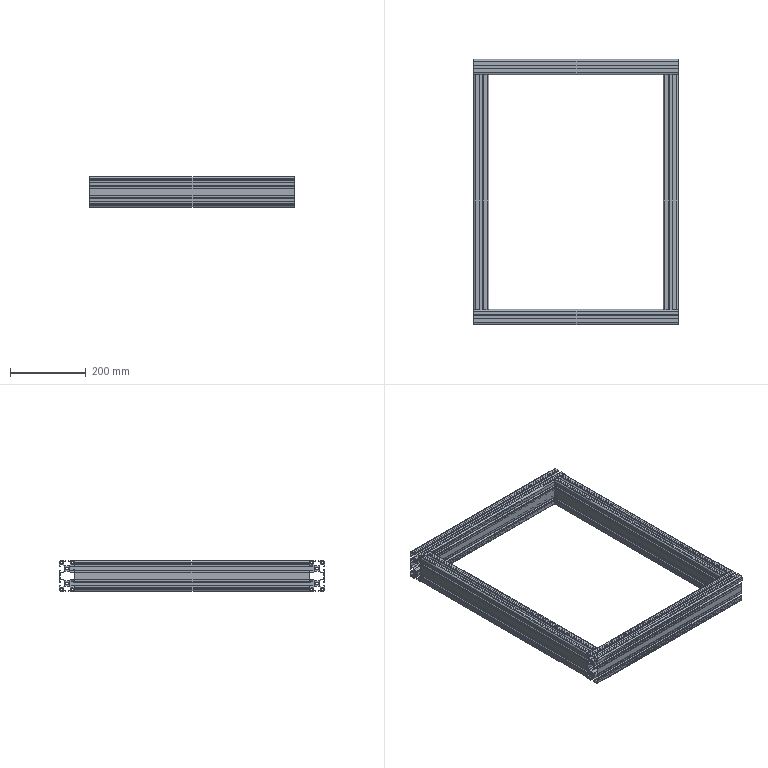Part | SolidWorks | features 3DProfileFeature 1, ICE 1, WeldCornerFeat 1, WeldMemberFeat 1, WeldmentFeature 1 | 5 solids | 982 faces | box 540.002 x 700.002 x 80 mm | volume 2304321 mm3 | plane 924 | cylinder 58 | commonest cylinder face diameters 9 x26 5 x16 6.8 x16